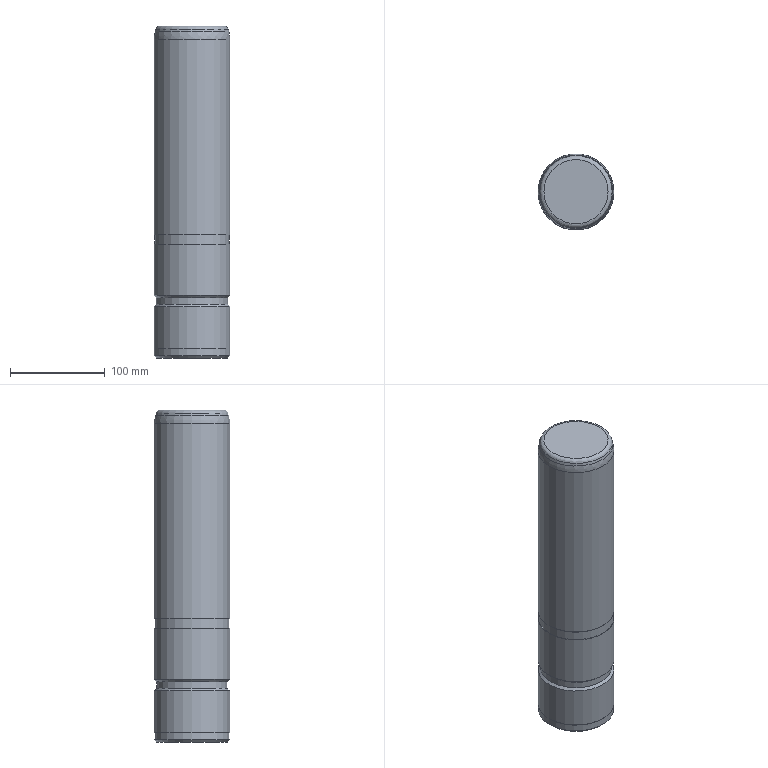Part | NX | features SGP 80-250 2 | 1 solid | 17 faces | box 80 x 80 x 350 mm | volume 1746865 mm3 | cylinder 6 | plane 5 | cone 4 | torus 2 | commonest cylinder face diameters 80 x3 75 x1 79 x1 79.5 x1
STEP:
#1=CARTESIAN_POINT('',(-1475.,-610.,-64.));
#2=VERTEX_POINT('',#1);
#3=CARTESIAN_POINT('',(-1435.,-610.,-64.));
#4=DIRECTION('',(0.,0.,1.));
#5=DIRECTION('',(-1.,0.,0.));
#6=AXIS2_PLACEMENT_3D('',#3,#4,#5);
#7=CIRCLE('',#6,40.);
#8=EDGE_CURVE('',#2,#2,#7,.F.);
#9=ORIENTED_EDGE('',*,*,#8,.F.);
#10=EDGE_LOOP('',(#9));
#11=FACE_BOUND('',#10,.T.);
#12=CARTESIAN_POINT('',(-1395.,-610.,-10.));
#13=VERTEX_POINT('',#12);
#14=CARTESIAN_POINT('',(-1435.,-610.,-10.));
#15=DIRECTION('',(0.,0.,-1.));
#16=DIRECTION('',(1.,0.,0.));
#17=AXIS2_PLACEMENT_3D('',#14,#15,#16);
#18=CIRCLE('',#17,40.);
#19=EDGE_CURVE('',#13,#13,#18,.T.);
#20=ORIENTED_EDGE('',*,*,#19,.T.);
#21=EDGE_LOOP('',(#20));
#22=FACE_BOUND('',#21,.T.);
#23=CARTESIAN_POINT('',(-1435.,-610.,-120.));
#24=DIRECTION('',(0.,0.,1.));
#25=DIRECTION('',(-1.,0.,0.));
#26=AXIS2_PLACEMENT_3D('',#23,#24,#25);
#27=CYLINDRICAL_SURFACE('',#26,40.);
#28=ADVANCED_FACE('',(#11,#22),#27,.T.);
#29=CARTESIAN_POINT('',(-1474.5,-610.,-10.));
#30=VERTEX_POINT('',#29);
#31=CARTESIAN_POINT('',(-1435.,-610.,-10.));
#32=DIRECTION('',(0.,0.,1.));
#33=DIRECTION('',(-1.,0.,0.));
#34=AXIS2_PLACEMENT_3D('',#31,#32,#33);
#35=CIRCLE('',#34,39.5);
#36=EDGE_CURVE('',#30,#30,#35,.T.);
#37=ORIENTED_EDGE('',*,*,#36,.F.);
#38=EDGE_LOOP('',(#37));
#39=FACE_BOUND('',#38,.T.);
#40=ORIENTED_EDGE('',*,*,#19,.F.);
#41=EDGE_LOOP('',(#40));
#42=FACE_BOUND('',#41,.T.);
#43=CARTESIAN_POINT('',(-1435.,-610.,-10.));
#44=DIRECTION('',(0.,0.,1.));
#45=DIRECTION('',(-1.,0.,0.));
#46=AXIS2_PLACEMENT_3D('',#43,#44,#45);
#47=PLANE('',#46);
#48=ADVANCED_FACE('',(#39,#42),#47,.T.);
#49=CARTESIAN_POINT('',(-1395.5,-610.,0.));
#50=VERTEX_POINT('',#49);
#51=CARTESIAN_POINT('',(-1435.,-610.,0.));
#52=DIRECTION('',(0.,0.,-1.));
#53=DIRECTION('',(1.,0.,0.));
#54=AXIS2_PLACEMENT_3D('',#51,#52,#53);
#55=CIRCLE('',#54,39.5);
#56=EDGE_CURVE('',#50,#50,#55,.F.);
#57=ORIENTED_EDGE('',*,*,#56,.F.);
#58=EDGE_LOOP('',(#57));
#59=FACE_BOUND('',#58,.T.);
#60=ORIENTED_EDGE('',*,*,#36,.T.);
#61=EDGE_LOOP('',(#60));
#62=FACE_BOUND('',#61,.T.);
#63=CARTESIAN_POINT('',(-1435.,-610.,-10.));
#64=DIRECTION('',(0.,0.,1.));
#65=DIRECTION('',(-1.,0.,0.));
#66=AXIS2_PLACEMENT_3D('',#63,#64,#65);
#67=CYLINDRICAL_SURFACE('',#66,39.5);
#68=ADVANCED_FACE('',(#59,#62),#67,.T.);
#69=ORIENTED_EDGE('',*,*,#56,.T.);
#70=EDGE_LOOP('',(#69));
#71=FACE_BOUND('',#70,.T.);
#72=CARTESIAN_POINT('',(-1475.,-610.,0.));
#73=VERTEX_POINT('',#72);
#74=CARTESIAN_POINT('',(-1435.,-610.,0.));
#75=DIRECTION('',(0.,0.,-1.));
#76=DIRECTION('',(-1.,0.,0.));
#77=AXIS2_PLACEMENT_3D('',#74,#75,#76);
#78=CIRCLE('',#77,40.);
#79=EDGE_CURVE('',#73,#73,#78,.F.);
#80=ORIENTED_EDGE('',*,*,#79,.F.);
#81=EDGE_LOOP('',(#80));
#82=FACE_BOUND('',#81,.T.);
#83=CARTESIAN_POINT('',(-1435.,-610.,0.));
#84=DIRECTION('',(0.,0.,-1.));
#85=DIRECTION('',(1.,0.,0.));
#86=AXIS2_PLACEMENT_3D('',#83,#84,#85);
#87=PLANE('',#86);
#88=ADVANCED_FACE('',(#71,#82),#87,.T.);
#89=CARTESIAN_POINT('',(-1395.,-610.,206.05));
#90=VERTEX_POINT('',#89);
#91=CARTESIAN_POINT('',(-1435.,-610.,206.05));
#92=DIRECTION('',(0.,0.,-1.));
#93=DIRECTION('',(1.,0.,0.));
#94=AXIS2_PLACEMENT_3D('',#91,#92,#93);
#95=CIRCLE('',#94,40.);
#96=EDGE_CURVE('',#90,#90,#95,.T.);
#97=ORIENTED_EDGE('',*,*,#96,.T.);
#98=EDGE_LOOP('',(#97));
#99=FACE_BOUND('',#98,.T.);
#100=ORIENTED_EDGE('',*,*,#79,.T.);
#101=EDGE_LOOP('',(#100));
#102=FACE_BOUND('',#101,.T.);
#103=CARTESIAN_POINT('',(-1435.,-610.,100.));
#104=DIRECTION('',(0.,0.,1.));
#105=DIRECTION('',(-1.,0.,0.));
#106=AXIS2_PLACEMENT_3D('',#103,#104,#105);
#107=CYLINDRICAL_SURFACE('',#106,40.);
#108=ADVANCED_FACE('',(#99,#102),#107,.T.);
#109=CARTESIAN_POINT('',(-1468.868,-610.,220.));
#110=VERTEX_POINT('',#109);
#111=CARTESIAN_POINT('',(-1435.,-610.,220.));
#112=DIRECTION('',(0.,0.,1.));
#113=DIRECTION('',(-1.,0.,0.));
#114=AXIS2_PLACEMENT_3D('',#111,#112,#113);
#115=CIRCLE('',#114,33.868);
#116=EDGE_CURVE('',#110,#110,#115,.T.);
#117=ORIENTED_EDGE('',*,*,#116,.T.);
#118=EDGE_LOOP('',(#117));
#119=FACE_BOUND('',#118,.T.);
#120=CARTESIAN_POINT('',(-1435.,-610.,220.));
#121=DIRECTION('',(0.,0.,1.));
#122=DIRECTION('',(-1.,0.,0.));
#123=AXIS2_PLACEMENT_3D('',#120,#121,#122);
#124=PLANE('',#123);
#125=ADVANCED_FACE('',(#119),#124,.T.);
#126=CARTESIAN_POINT('',(-1473.214,-610.,216.665));
#127=VERTEX_POINT('',#126);
#128=CARTESIAN_POINT('',(-1435.,-610.,216.665));
#129=DIRECTION('',(0.,0.,1.));
#130=DIRECTION('',(-1.,0.,0.));
#131=AXIS2_PLACEMENT_3D('',#128,#129,#130);
#132=CIRCLE('',#131,38.214);
#133=EDGE_CURVE('',#127,#127,#132,.F.);
#134=ORIENTED_EDGE('',*,*,#133,.T.);
#135=EDGE_LOOP('',(#134));
#136=FACE_BOUND('',#135,.T.);
#137=CARTESIAN_POINT('',(-1473.978,-610.,213.815));
#138=VERTEX_POINT('',#137);
#139=CARTESIAN_POINT('',(-1435.,-610.,213.815));
#140=DIRECTION('',(0.,0.,1.));
#141=DIRECTION('',(-1.,0.,0.));
#142=AXIS2_PLACEMENT_3D('',#139,#140,#141);
#143=CIRCLE('',#142,38.978);
#144=EDGE_CURVE('',#138,#138,#143,.T.);
#145=ORIENTED_EDGE('',*,*,#144,.T.);
#146=EDGE_LOOP('',(#145));
#147=FACE_BOUND('',#146,.T.);
#148=CARTESIAN_POINT('',(-1435.,-610.,220.));
#149=DIRECTION('',(0.,0.,-1.));
#150=DIRECTION('',(1.,0.,0.));
#151=AXIS2_PLACEMENT_3D('',#148,#149,#150);
#152=CONICAL_SURFACE('',#151,37.321,0.2618);
#153=ADVANCED_FACE('',(#136,#147),#152,.T.);
#154=CARTESIAN_POINT('',(-1472.5,-610.,-66.5));
#155=VERTEX_POINT('',#154);
#156=CARTESIAN_POINT('',(-1435.,-610.,-66.5));
#157=DIRECTION('',(0.,0.,1.));
#158=DIRECTION('',(-1.,0.,0.));
#159=AXIS2_PLACEMENT_3D('',#156,#157,#158);
#160=CIRCLE('',#159,37.5);
#161=EDGE_CURVE('',#155,#155,#160,.F.);
#162=ORIENTED_EDGE('',*,*,#161,.T.);
#163=EDGE_LOOP('',(#162));
#164=FACE_BOUND('',#163,.T.);
#165=CARTESIAN_POINT('',(-1397.5,-610.,-73.5));
#166=VERTEX_POINT('',#165);
#167=CARTESIAN_POINT('',(-1435.,-610.,-73.5));
#168=DIRECTION('',(0.,0.,-1.));
#169=DIRECTION('',(1.,0.,0.));
#170=AXIS2_PLACEMENT_3D('',#167,#168,#169);
#171=CIRCLE('',#170,37.5);
#172=EDGE_CURVE('',#166,#166,#171,.F.);
#173=ORIENTED_EDGE('',*,*,#172,.T.);
#174=EDGE_LOOP('',(#173));
#175=FACE_BOUND('',#174,.T.);
#176=CARTESIAN_POINT('',(-1435.,-610.,-76.));
#177=DIRECTION('',(0.,0.,1.));
#178=DIRECTION('',(-1.,0.,0.));
#179=AXIS2_PLACEMENT_3D('',#176,#177,#178);
#180=CYLINDRICAL_SURFACE('',#179,37.5);
#181=ADVANCED_FACE('',(#164,#175),#180,.T.);
#182=CARTESIAN_POINT('',(-1397.75,-610.,-130.));
#183=VERTEX_POINT('',#182);
#184=CARTESIAN_POINT('',(-1435.,-610.,-130.));
#185=DIRECTION('',(0.,0.,-1.));
#186=DIRECTION('',(1.,0.,0.));
#187=AXIS2_PLACEMENT_3D('',#184,#185,#186);
#188=CIRCLE('',#187,37.25);
#189=EDGE_CURVE('',#183,#183,#188,.T.);
#190=ORIENTED_EDGE('',*,*,#189,.T.);
#191=EDGE_LOOP('',(#190));
#192=FACE_BOUND('',#191,.T.);
#193=CARTESIAN_POINT('',(-1435.,-610.,-130.));
#194=DIRECTION('',(0.,0.,-1.));
#195=DIRECTION('',(1.,0.,0.));
#196=AXIS2_PLACEMENT_3D('',#193,#194,#195);
#197=PLANE('',#196);
#198=ADVANCED_FACE('',(#192),#197,.T.);
#199=CARTESIAN_POINT('',(-1395.25,-610.,-127.5));
#200=VERTEX_POINT('',#199);
#201=CARTESIAN_POINT('',(-1435.,-610.,-127.5));
#202=DIRECTION('',(0.,0.,-1.));
#203=DIRECTION('',(1.,0.,0.));
#204=AXIS2_PLACEMENT_3D('',#201,#202,#203);
#205=CIRCLE('',#204,39.75);
#206=EDGE_CURVE('',#200,#200,#205,.F.);
#207=ORIENTED_EDGE('',*,*,#206,.T.);
#208=EDGE_LOOP('',(#207));
#209=FACE_BOUND('',#208,.T.);
#210=CARTESIAN_POINT('',(-1395.25,-610.,-120.));
#211=VERTEX_POINT('',#210);
#212=CARTESIAN_POINT('',(-1435.,-610.,-120.));
#213=DIRECTION('',(0.,0.,-1.));
#214=DIRECTION('',(1.,0.,0.));
#215=AXIS2_PLACEMENT_3D('',#212,#213,#214);
#216=CIRCLE('',#215,39.75);
#217=EDGE_CURVE('',#211,#211,#216,.F.);
#218=ORIENTED_EDGE('',*,*,#217,.F.);
#219=EDGE_LOOP('',(#218));
#220=FACE_BOUND('',#219,.T.);
#221=CARTESIAN_POINT('',(-1435.,-610.,-130.));
#222=DIRECTION('',(0.,0.,1.));
#223=DIRECTION('',(-1.,0.,0.));
#224=AXIS2_PLACEMENT_3D('',#221,#222,#223);
#225=CYLINDRICAL_SURFACE('',#224,39.75);
#226=ADVANCED_FACE('',(#209,#220),#225,.T.);
#227=ORIENTED_EDGE('',*,*,#217,.T.);
#228=EDGE_LOOP('',(#227));
#229=FACE_BOUND('',#228,.T.);
#230=CARTESIAN_POINT('',(-1475.,-610.,-120.));
#231=VERTEX_POINT('',#230);
#232=CARTESIAN_POINT('',(-1435.,-610.,-120.));
#233=DIRECTION('',(0.,0.,1.));
#234=DIRECTION('',(-1.,0.,0.));
#235=AXIS2_PLACEMENT_3D('',#232,#233,#234);
#236=CIRCLE('',#235,40.);
#237=EDGE_CURVE('',#231,#231,#236,.T.);
#238=ORIENTED_EDGE('',*,*,#237,.F.);
#239=EDGE_LOOP('',(#238));
#240=FACE_BOUND('',#239,.T.);
#241=CARTESIAN_POINT('',(-1435.,-610.,-120.));
#242=DIRECTION('',(0.,0.,-1.));
#243=DIRECTION('',(1.,0.,0.));
#244=AXIS2_PLACEMENT_3D('',#241,#242,#243);
#245=PLANE('',#244);
#246=ADVANCED_FACE('',(#229,#240),#245,.T.);
#247=CARTESIAN_POINT('',(-1395.,-610.,-76.));
#248=VERTEX_POINT('',#247);
#249=CARTESIAN_POINT('',(-1435.,-610.,-76.));
#250=DIRECTION('',(0.,0.,-1.));
#251=DIRECTION('',(1.,0.,0.));
#252=AXIS2_PLACEMENT_3D('',#249,#250,#251);
#253=CIRCLE('',#252,40.);
#254=EDGE_CURVE('',#248,#248,#253,.F.);
#255=ORIENTED_EDGE('',*,*,#254,.F.);
#256=EDGE_LOOP('',(#255));
#257=FACE_BOUND('',#256,.T.);
#258=ORIENTED_EDGE('',*,*,#237,.T.);
#259=EDGE_LOOP('',(#258));
#260=FACE_BOUND('',#259,.T.);
#261=CARTESIAN_POINT('',(-1435.,-610.,-120.));
#262=DIRECTION('',(0.,0.,1.));
#263=DIRECTION('',(-1.,0.,0.));
#264=AXIS2_PLACEMENT_3D('',#261,#262,#263);
#265=CYLINDRICAL_SURFACE('',#264,40.);
#266=ADVANCED_FACE('',(#257,#260),#265,.T.);
#267=ORIENTED_EDGE('',*,*,#189,.F.);
#268=EDGE_LOOP('',(#267));
#269=FACE_BOUND('',#268,.T.);
#270=ORIENTED_EDGE('',*,*,#206,.F.);
#271=EDGE_LOOP('',(#270));
#272=FACE_BOUND('',#271,.T.);
#273=CARTESIAN_POINT('',(-1435.,-610.,-127.5));
#274=DIRECTION('',(0.,0.,1.));
#275=DIRECTION('',(-1.,0.,0.));
#276=AXIS2_PLACEMENT_3D('',#273,#274,#275);
#277=CONICAL_SURFACE('',#276,39.75,0.7854);
#278=ADVANCED_FACE('',(#269,#272),#277,.T.);
#279=ORIENTED_EDGE('',*,*,#254,.T.);
#280=EDGE_LOOP('',(#279));
#281=FACE_BOUND('',#280,.T.);
#282=ORIENTED_EDGE('',*,*,#172,.F.);
#283=EDGE_LOOP('',(#282));
#284=FACE_BOUND('',#283,.T.);
#285=CARTESIAN_POINT('',(-1435.,-610.,-73.5));
#286=DIRECTION('',(0.,0.,-1.));
#287=DIRECTION('',(1.,0.,0.));
#288=AXIS2_PLACEMENT_3D('',#285,#286,#287);
#289=CONICAL_SURFACE('',#288,37.5,0.7854);
#290=ADVANCED_FACE('',(#281,#284),#289,.T.);
#291=ORIENTED_EDGE('',*,*,#8,.T.);
#292=EDGE_LOOP('',(#291));
#293=FACE_BOUND('',#292,.T.);
#294=ORIENTED_EDGE('',*,*,#161,.F.);
#295=EDGE_LOOP('',(#294));
#296=FACE_BOUND('',#295,.T.);
#297=CARTESIAN_POINT('',(-1435.,-610.,-66.5));
#298=DIRECTION('',(0.,0.,1.));
#299=DIRECTION('',(-1.,0.,0.));
#300=AXIS2_PLACEMENT_3D('',#297,#298,#299);
#301=CONICAL_SURFACE('',#300,37.5,0.7854);
#302=ADVANCED_FACE('',(#293,#296),#301,.T.);
#303=ORIENTED_EDGE('',*,*,#96,.F.);
#304=EDGE_LOOP('',(#303));
#305=FACE_BOUND('',#304,.T.);
#306=ORIENTED_EDGE('',*,*,#144,.F.);
#307=EDGE_LOOP('',(#306));
#308=FACE_BOUND('',#307,.T.);
#309=CARTESIAN_POINT('',(-1435.,-610.,206.05));
#310=DIRECTION('',(0.,0.,-1.));
#311=DIRECTION('',(1.,0.,0.));
#312=AXIS2_PLACEMENT_3D('',#309,#310,#311);
#313=DEGENERATE_TOROIDAL_SURFACE('',#312,10.,30.,.T.);
#314=ADVANCED_FACE('',(#305,#308),#313,.T.);
#315=ORIENTED_EDGE('',*,*,#116,.F.);
#316=EDGE_LOOP('',(#315));
#317=FACE_BOUND('',#316,.T.);
#318=ORIENTED_EDGE('',*,*,#133,.F.);
#319=EDGE_LOOP('',(#318));
#320=FACE_BOUND('',#319,.T.);
#321=CARTESIAN_POINT('',(-1435.,-610.,215.5));
#322=DIRECTION('',(0.,0.,1.));
#323=DIRECTION('',(-1.,0.,0.));
#324=AXIS2_PLACEMENT_3D('',#321,#322,#323);
#325=TOROIDAL_SURFACE('',#324,33.868,4.5);
#326=ADVANCED_FACE('',(#317,#320),#325,.T.);
#327=CLOSED_SHELL('',(#28,#48,#68,#88,#108,#125,#153,#181,#198,#226,#246,#266,#278,#290,#302,#314,#326));
#328=MANIFOLD_SOLID_BREP('',#327);
#329=(LENGTH_UNIT()NAMED_UNIT(*)SI_UNIT(.MILLI.,.METRE.));
#330=UNCERTAINTY_MEASURE_WITH_UNIT(LENGTH_MEASURE(0.00001),#329,'','');
#331=(NAMED_UNIT(*)PLANE_ANGLE_UNIT()SI_UNIT($,.RADIAN.));
#332=(NAMED_UNIT(*)SI_UNIT($,.STERADIAN.)SOLID_ANGLE_UNIT());
#333=(GEOMETRIC_REPRESENTATION_CONTEXT(3)GLOBAL_UNCERTAINTY_ASSIGNED_CONTEXT((#330))GLOBAL_UNIT_ASSIGNED_CONTEXT((#329,#331,#332))REPRESENTATION_CONTEXT('',''));
#334=ADVANCED_BREP_SHAPE_REPRESENTATION('',(#328),#333);